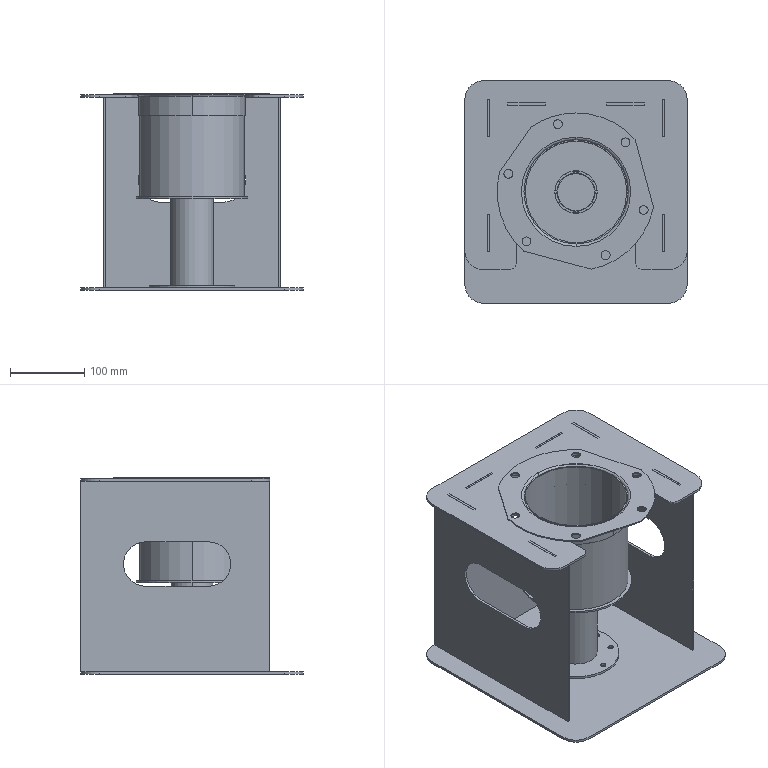Part | SolidWorks | features MirrorCompFeat 1, ReferencePattern 1 | 10 solids | 247 faces | box 300 x 300 x 265.3 mm | volume 1237599 mm3 | plane 151 | cylinder 92 | torus 4 | commonest cylinder face diameters 7.2 x24 12 x20 50 x10 60 x7 4 x6 213 x4